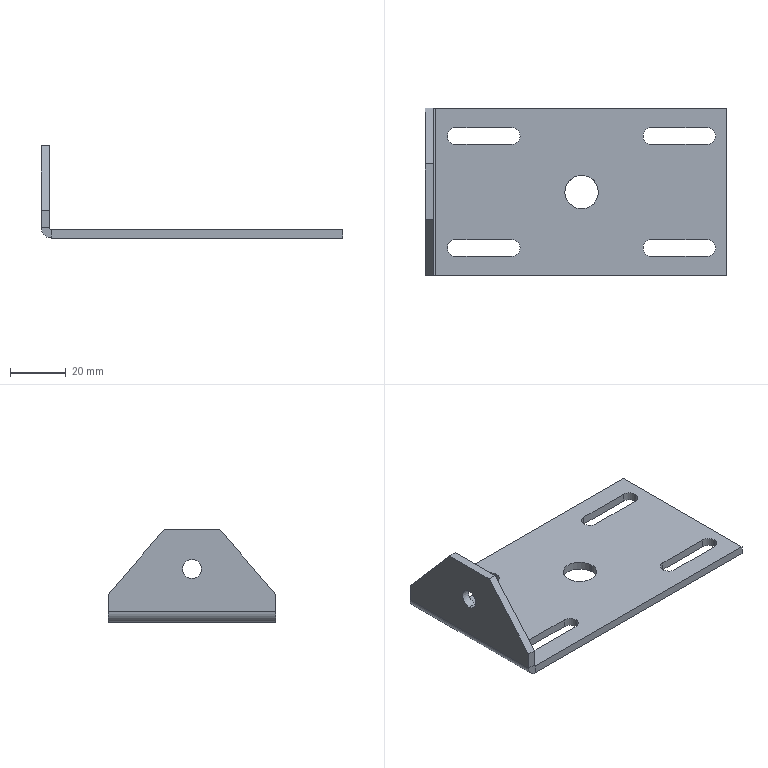Part | NX | features BREP 1 | 1 solid | 40 faces | box 108 x 60 x 33 mm | volume 21060 mm3 | plane 22 | cylinder 18 | commonest cylinder face diameters 6 x12 6.8 x2 12 x2 1.473 x1 7.473 x1
STEP:
#1=CARTESIAN_POINT('',(-48.,0.,12.6));
#2=VERTEX_POINT('',#1);
#3=CARTESIAN_POINT('',(-45.,0.,12.6));
#4=VERTEX_POINT('',#3);
#5=CARTESIAN_POINT('',(-48.,0.,12.6));
#6=DIRECTION('',(-1.,0.,0.));
#7=VECTOR('',#6,1000.);
#8=LINE('',#5,#7);
#9=EDGE_CURVE('',#2,#4,#8,.F.);
#10=ORIENTED_EDGE('',*,*,#9,.T.);
#11=CARTESIAN_POINT('',(-45.,0.,19.4));
#12=VERTEX_POINT('',#11);
#13=CARTESIAN_POINT('',(-45.,0.,16.));
#14=DIRECTION('',(1.,0.,0.));
#15=DIRECTION('',(0.,0.,-1.));
#16=AXIS2_PLACEMENT_3D('',#13,#14,#15);
#17=CIRCLE('',#16,3.4);
#18=EDGE_CURVE('',#4,#12,#17,.T.);
#19=ORIENTED_EDGE('',*,*,#18,.T.);
#20=CARTESIAN_POINT('',(-48.,0.,19.4));
#21=VERTEX_POINT('',#20);
#22=CARTESIAN_POINT('',(-48.,0.,19.4));
#23=DIRECTION('',(-1.,0.,0.));
#24=VECTOR('',#23,1000.);
#25=LINE('',#22,#24);
#26=EDGE_CURVE('',#21,#12,#25,.F.);
#27=ORIENTED_EDGE('',*,*,#26,.F.);
#28=CARTESIAN_POINT('',(-48.,0.,16.));
#29=DIRECTION('',(-1.,0.,0.));
#30=DIRECTION('',(0.,0.,1.));
#31=AXIS2_PLACEMENT_3D('',#28,#29,#30);
#32=CIRCLE('',#31,3.4);
#33=EDGE_CURVE('',#21,#2,#32,.T.);
#34=ORIENTED_EDGE('',*,*,#33,.T.);
#35=EDGE_LOOP('',(#10,#19,#27,#34));
#36=FACE_BOUND('',#35,.T.);
#37=CARTESIAN_POINT('',(-48.,0.,16.));
#38=DIRECTION('',(-1.,0.,0.));
#39=DIRECTION('',(0.,0.,1.));
#40=AXIS2_PLACEMENT_3D('',#37,#38,#39);
#41=CYLINDRICAL_SURFACE('',#40,3.4);
#42=ADVANCED_FACE('',(#36),#41,.F.);
#43=CARTESIAN_POINT('',(-17.,-17.,-3.));
#44=VERTEX_POINT('',#43);
#45=CARTESIAN_POINT('',(-17.,-17.,0.));
#46=VERTEX_POINT('',#45);
#47=CARTESIAN_POINT('',(-17.,-17.,-10.));
#48=DIRECTION('',(0.,0.,1.));
#49=VECTOR('',#48,1000.);
#50=LINE('',#47,#49);
#51=EDGE_CURVE('',#44,#46,#50,.T.);
#52=ORIENTED_EDGE('',*,*,#51,.T.);
#53=CARTESIAN_POINT('',(-37.,-17.,0.));
#54=VERTEX_POINT('',#53);
#55=CARTESIAN_POINT('',(-17.,-17.,0.));
#56=DIRECTION('',(-1.,0.,0.));
#57=VECTOR('',#56,1000.);
#58=LINE('',#55,#57);
#59=EDGE_CURVE('',#46,#54,#58,.T.);
#60=ORIENTED_EDGE('',*,*,#59,.T.);
#61=CARTESIAN_POINT('',(-37.,-17.,-3.));
#62=VERTEX_POINT('',#61);
#63=CARTESIAN_POINT('',(-37.,-17.,-10.));
#64=DIRECTION('',(0.,0.,1.));
#65=VECTOR('',#64,1000.);
#66=LINE('',#63,#65);
#67=EDGE_CURVE('',#62,#54,#66,.T.);
#68=ORIENTED_EDGE('',*,*,#67,.F.);
#69=CARTESIAN_POINT('',(0.,-17.,-3.));
#70=DIRECTION('',(-1.,0.,0.));
#71=VECTOR('',#70,1000.);
#72=LINE('',#69,#71);
#73=EDGE_CURVE('',#44,#62,#72,.T.);
#74=ORIENTED_EDGE('',*,*,#73,.F.);
#75=EDGE_LOOP('',(#52,#60,#68,#74));
#76=FACE_BOUND('',#75,.T.);
#77=CARTESIAN_POINT('',(-17.,-17.,-10.));
#78=DIRECTION('',(0.,1.,0.));
#79=DIRECTION('',(-1.,0.,0.));
#80=AXIS2_PLACEMENT_3D('',#77,#78,#79);
#81=PLANE('',#80);
#82=ADVANCED_FACE('',(#76),#81,.F.);
#83=ORIENTED_EDGE('',*,*,#67,.T.);
#84=CARTESIAN_POINT('',(-37.,-23.,0.));
#85=VERTEX_POINT('',#84);
#86=CARTESIAN_POINT('',(-37.,-20.,0.));
#87=DIRECTION('',(0.,0.,1.));
#88=DIRECTION('',(1.,0.,0.));
#89=AXIS2_PLACEMENT_3D('',#86,#87,#88);
#90=CIRCLE('',#89,3.);
#91=EDGE_CURVE('',#54,#85,#90,.T.);
#92=ORIENTED_EDGE('',*,*,#91,.T.);
#93=CARTESIAN_POINT('',(-37.,-23.,-3.));
#94=VERTEX_POINT('',#93);
#95=CARTESIAN_POINT('',(-37.,-23.,-10.));
#96=DIRECTION('',(0.,0.,1.));
#97=VECTOR('',#96,1000.);
#98=LINE('',#95,#97);
#99=EDGE_CURVE('',#94,#85,#98,.T.);
#100=ORIENTED_EDGE('',*,*,#99,.F.);
#101=CARTESIAN_POINT('',(-37.,-20.,-3.));
#102=DIRECTION('',(0.,0.,1.));
#103=DIRECTION('',(1.,0.,0.));
#104=AXIS2_PLACEMENT_3D('',#101,#102,#103);
#105=CIRCLE('',#104,3.);
#106=EDGE_CURVE('',#62,#94,#105,.T.);
#107=ORIENTED_EDGE('',*,*,#106,.F.);
#108=EDGE_LOOP('',(#83,#92,#100,#107));
#109=FACE_BOUND('',#108,.T.);
#110=CARTESIAN_POINT('',(-37.,-20.,-10.));
#111=DIRECTION('',(0.,0.,1.));
#112=DIRECTION('',(1.,0.,0.));
#113=AXIS2_PLACEMENT_3D('',#110,#111,#112);
#114=CYLINDRICAL_SURFACE('',#113,3.);
#115=ADVANCED_FACE('',(#109),#114,.F.);
#116=ORIENTED_EDGE('',*,*,#99,.T.);
#117=CARTESIAN_POINT('',(-17.,-23.,0.));
#118=VERTEX_POINT('',#117);
#119=CARTESIAN_POINT('',(-17.,-23.,0.));
#120=DIRECTION('',(1.,0.,0.));
#121=VECTOR('',#120,1000.);
#122=LINE('',#119,#121);
#123=EDGE_CURVE('',#85,#118,#122,.T.);
#124=ORIENTED_EDGE('',*,*,#123,.T.);
#125=CARTESIAN_POINT('',(-17.,-23.,-3.));
#126=VERTEX_POINT('',#125);
#127=CARTESIAN_POINT('',(-17.,-23.,-10.));
#128=DIRECTION('',(0.,0.,1.));
#129=VECTOR('',#128,1000.);
#130=LINE('',#127,#129);
#131=EDGE_CURVE('',#126,#118,#130,.T.);
#132=ORIENTED_EDGE('',*,*,#131,.F.);
#133=CARTESIAN_POINT('',(0.,-23.,-3.));
#134=DIRECTION('',(1.,0.,0.));
#135=VECTOR('',#134,1000.);
#136=LINE('',#133,#135);
#137=EDGE_CURVE('',#94,#126,#136,.T.);
#138=ORIENTED_EDGE('',*,*,#137,.F.);
#139=EDGE_LOOP('',(#116,#124,#132,#138));
#140=FACE_BOUND('',#139,.T.);
#141=CARTESIAN_POINT('',(-17.,-23.,-10.));
#142=DIRECTION('',(0.,-1.,0.));
#143=DIRECTION('',(1.,0.,0.));
#144=AXIS2_PLACEMENT_3D('',#141,#142,#143);
#145=PLANE('',#144);
#146=ADVANCED_FACE('',(#140),#145,.F.);
#147=CARTESIAN_POINT('',(-14.,-20.,-3.));
#148=VERTEX_POINT('',#147);
#149=CARTESIAN_POINT('',(-14.,-20.,0.));
#150=VERTEX_POINT('',#149);
#151=CARTESIAN_POINT('',(-14.,-20.,-10.));
#152=DIRECTION('',(0.,0.,1.));
#153=VECTOR('',#152,1000.);
#154=LINE('',#151,#153);
#155=EDGE_CURVE('',#148,#150,#154,.T.);
#156=ORIENTED_EDGE('',*,*,#155,.F.);
#157=CARTESIAN_POINT('',(-17.,-20.,-3.));
#158=DIRECTION('',(0.,0.,1.));
#159=DIRECTION('',(1.,0.,0.));
#160=AXIS2_PLACEMENT_3D('',#157,#158,#159);
#161=CIRCLE('',#160,3.);
#162=EDGE_CURVE('',#126,#148,#161,.T.);
#163=ORIENTED_EDGE('',*,*,#162,.F.);
#164=ORIENTED_EDGE('',*,*,#131,.T.);
#165=CARTESIAN_POINT('',(-17.,-20.,0.));
#166=DIRECTION('',(0.,0.,1.));
#167=DIRECTION('',(1.,0.,0.));
#168=AXIS2_PLACEMENT_3D('',#165,#166,#167);
#169=CIRCLE('',#168,3.);
#170=EDGE_CURVE('',#118,#150,#169,.T.);
#171=ORIENTED_EDGE('',*,*,#170,.T.);
#172=EDGE_LOOP('',(#156,#163,#164,#171));
#173=FACE_BOUND('',#172,.T.);
#174=CARTESIAN_POINT('',(-17.,-20.,-10.));
#175=DIRECTION('',(0.,0.,1.));
#176=DIRECTION('',(1.,0.,0.));
#177=AXIS2_PLACEMENT_3D('',#174,#175,#176);
#178=CYLINDRICAL_SURFACE('',#177,3.);
#179=ADVANCED_FACE('',(#173),#178,.F.);
#180=CARTESIAN_POINT('',(33.,-23.,-3.));
#181=VERTEX_POINT('',#180);
#182=CARTESIAN_POINT('',(33.,-23.,0.));
#183=VERTEX_POINT('',#182);
#184=CARTESIAN_POINT('',(33.,-23.,-10.));
#185=DIRECTION('',(0.,0.,1.));
#186=VECTOR('',#185,1000.);
#187=LINE('',#184,#186);
#188=EDGE_CURVE('',#181,#183,#187,.T.);
#189=ORIENTED_EDGE('',*,*,#188,.T.);
#190=CARTESIAN_POINT('',(53.,-23.,0.));
#191=VERTEX_POINT('',#190);
#192=CARTESIAN_POINT('',(33.,-23.,0.));
#193=DIRECTION('',(1.,0.,0.));
#194=VECTOR('',#193,1000.);
#195=LINE('',#192,#194);
#196=EDGE_CURVE('',#183,#191,#195,.T.);
#197=ORIENTED_EDGE('',*,*,#196,.T.);
#198=CARTESIAN_POINT('',(53.,-23.,-3.));
#199=VERTEX_POINT('',#198);
#200=CARTESIAN_POINT('',(53.,-23.,-10.));
#201=DIRECTION('',(0.,0.,1.));
#202=VECTOR('',#201,1000.);
#203=LINE('',#200,#202);
#204=EDGE_CURVE('',#199,#191,#203,.T.);
#205=ORIENTED_EDGE('',*,*,#204,.F.);
#206=CARTESIAN_POINT('',(0.,-23.,-3.));
#207=DIRECTION('',(1.,0.,0.));
#208=VECTOR('',#207,1000.);
#209=LINE('',#206,#208);
#210=EDGE_CURVE('',#181,#199,#209,.T.);
#211=ORIENTED_EDGE('',*,*,#210,.F.);
#212=EDGE_LOOP('',(#189,#197,#205,#211));
#213=FACE_BOUND('',#212,.T.);
#214=CARTESIAN_POINT('',(33.,-23.,-10.));
#215=DIRECTION('',(0.,-1.,0.));
#216=DIRECTION('',(1.,0.,0.));
#217=AXIS2_PLACEMENT_3D('',#214,#215,#216);
#218=PLANE('',#217);
#219=ADVANCED_FACE('',(#213),#218,.F.);
#220=CARTESIAN_POINT('',(56.,-20.,-3.));
#221=VERTEX_POINT('',#220);
#222=CARTESIAN_POINT('',(56.,-20.,0.));
#223=VERTEX_POINT('',#222);
#224=CARTESIAN_POINT('',(56.,-20.,-10.));
#225=DIRECTION('',(0.,0.,1.));
#226=VECTOR('',#225,1000.);
#227=LINE('',#224,#226);
#228=EDGE_CURVE('',#221,#223,#227,.T.);
#229=ORIENTED_EDGE('',*,*,#228,.F.);
#230=CARTESIAN_POINT('',(53.,-20.,-3.));
#231=DIRECTION('',(0.,0.,1.));
#232=DIRECTION('',(1.,0.,0.));
#233=AXIS2_PLACEMENT_3D('',#230,#231,#232);
#234=CIRCLE('',#233,3.);
#235=EDGE_CURVE('',#199,#221,#234,.T.);
#236=ORIENTED_EDGE('',*,*,#235,.F.);
#237=ORIENTED_EDGE('',*,*,#204,.T.);
#238=CARTESIAN_POINT('',(53.,-20.,0.));
#239=DIRECTION('',(0.,0.,1.));
#240=DIRECTION('',(1.,0.,0.));
#241=AXIS2_PLACEMENT_3D('',#238,#239,#240);
#242=CIRCLE('',#241,3.);
#243=EDGE_CURVE('',#191,#223,#242,.T.);
#244=ORIENTED_EDGE('',*,*,#243,.T.);
#245=EDGE_LOOP('',(#229,#236,#237,#244));
#246=FACE_BOUND('',#245,.T.);
#247=CARTESIAN_POINT('',(53.,-20.,-10.));
#248=DIRECTION('',(0.,0.,1.));
#249=DIRECTION('',(1.,0.,0.));
#250=AXIS2_PLACEMENT_3D('',#247,#248,#249);
#251=CYLINDRICAL_SURFACE('',#250,3.);
#252=ADVANCED_FACE('',(#246),#251,.F.);
#253=CARTESIAN_POINT('',(53.,-17.,-3.));
#254=VERTEX_POINT('',#253);
#255=CARTESIAN_POINT('',(53.,-17.,0.));
#256=VERTEX_POINT('',#255);
#257=CARTESIAN_POINT('',(53.,-17.,-10.));
#258=DIRECTION('',(0.,0.,1.));
#259=VECTOR('',#258,1000.);
#260=LINE('',#257,#259);
#261=EDGE_CURVE('',#254,#256,#260,.T.);
#262=ORIENTED_EDGE('',*,*,#261,.T.);
#263=CARTESIAN_POINT('',(33.,-17.,0.));
#264=VERTEX_POINT('',#263);
#265=CARTESIAN_POINT('',(33.,-17.,0.));
#266=DIRECTION('',(-1.,0.,0.));
#267=VECTOR('',#266,1000.);
#268=LINE('',#265,#267);
#269=EDGE_CURVE('',#256,#264,#268,.T.);
#270=ORIENTED_EDGE('',*,*,#269,.T.);
#271=CARTESIAN_POINT('',(33.,-17.,-3.));
#272=VERTEX_POINT('',#271);
#273=CARTESIAN_POINT('',(33.,-17.,-10.));
#274=DIRECTION('',(0.,0.,1.));
#275=VECTOR('',#274,1000.);
#276=LINE('',#273,#275);
#277=EDGE_CURVE('',#272,#264,#276,.T.);
#278=ORIENTED_EDGE('',*,*,#277,.F.);
#279=CARTESIAN_POINT('',(0.,-17.,-3.));
#280=DIRECTION('',(-1.,0.,0.));
#281=VECTOR('',#280,1000.);
#282=LINE('',#279,#281);
#283=EDGE_CURVE('',#254,#272,#282,.T.);
#284=ORIENTED_EDGE('',*,*,#283,.F.);
#285=EDGE_LOOP('',(#262,#270,#278,#284));
#286=FACE_BOUND('',#285,.T.);
#287=CARTESIAN_POINT('',(33.,-17.,-10.));
#288=DIRECTION('',(0.,1.,0.));
#289=DIRECTION('',(-1.,0.,0.));
#290=AXIS2_PLACEMENT_3D('',#287,#288,#289);
#291=PLANE('',#290);
#292=ADVANCED_FACE('',(#286),#291,.F.);
#293=ORIENTED_EDGE('',*,*,#277,.T.);
#294=CARTESIAN_POINT('',(33.,-20.,0.));
#295=DIRECTION('',(0.,0.,1.));
#296=DIRECTION('',(1.,0.,0.));
#297=AXIS2_PLACEMENT_3D('',#294,#295,#296);
#298=CIRCLE('',#297,3.);
#299=EDGE_CURVE('',#264,#183,#298,.T.);
#300=ORIENTED_EDGE('',*,*,#299,.T.);
#301=ORIENTED_EDGE('',*,*,#188,.F.);
#302=CARTESIAN_POINT('',(33.,-20.,-3.));
#303=DIRECTION('',(0.,0.,1.));
#304=DIRECTION('',(1.,0.,0.));
#305=AXIS2_PLACEMENT_3D('',#302,#303,#304);
#306=CIRCLE('',#305,3.);
#307=EDGE_CURVE('',#272,#181,#306,.T.);
#308=ORIENTED_EDGE('',*,*,#307,.F.);
#309=EDGE_LOOP('',(#293,#300,#301,#308));
#310=FACE_BOUND('',#309,.T.);
#311=CARTESIAN_POINT('',(33.,-20.,-10.));
#312=DIRECTION('',(0.,0.,1.));
#313=DIRECTION('',(1.,0.,0.));
#314=AXIS2_PLACEMENT_3D('',#311,#312,#313);
#315=CYLINDRICAL_SURFACE('',#314,3.);
#316=ADVANCED_FACE('',(#310),#315,.F.);
#317=CARTESIAN_POINT('',(33.,17.,-3.));
#318=VERTEX_POINT('',#317);
#319=CARTESIAN_POINT('',(33.,17.,0.));
#320=VERTEX_POINT('',#319);
#321=CARTESIAN_POINT('',(33.,17.,-10.));
#322=DIRECTION('',(0.,0.,1.));
#323=VECTOR('',#322,1000.);
#324=LINE('',#321,#323);
#325=EDGE_CURVE('',#318,#320,#324,.T.);
#326=ORIENTED_EDGE('',*,*,#325,.T.);
#327=CARTESIAN_POINT('',(53.,17.,0.));
#328=VERTEX_POINT('',#327);
#329=CARTESIAN_POINT('',(33.,17.,0.));
#330=DIRECTION('',(1.,0.,0.));
#331=VECTOR('',#330,1000.);
#332=LINE('',#329,#331);
#333=EDGE_CURVE('',#320,#328,#332,.T.);
#334=ORIENTED_EDGE('',*,*,#333,.T.);
#335=CARTESIAN_POINT('',(53.,17.,-3.));
#336=VERTEX_POINT('',#335);
#337=CARTESIAN_POINT('',(53.,17.,-10.));
#338=DIRECTION('',(0.,0.,1.));
#339=VECTOR('',#338,1000.);
#340=LINE('',#337,#339);
#341=EDGE_CURVE('',#336,#328,#340,.T.);
#342=ORIENTED_EDGE('',*,*,#341,.F.);
#343=CARTESIAN_POINT('',(0.,17.,-3.));
#344=DIRECTION('',(1.,0.,0.));
#345=VECTOR('',#344,1000.);
#346=LINE('',#343,#345);
#347=EDGE_CURVE('',#318,#336,#346,.T.);
#348=ORIENTED_EDGE('',*,*,#347,.F.);
#349=EDGE_LOOP('',(#326,#334,#342,#348));
#350=FACE_BOUND('',#349,.T.);
#351=CARTESIAN_POINT('',(33.,17.,-10.));
#352=DIRECTION('',(0.,-1.,0.));
#353=DIRECTION('',(1.,0.,0.));
#354=AXIS2_PLACEMENT_3D('',#351,#352,#353);
#355=PLANE('',#354);
#356=ADVANCED_FACE('',(#350),#355,.F.);
#357=CARTESIAN_POINT('',(56.,20.,-3.));
#358=VERTEX_POINT('',#357);
#359=CARTESIAN_POINT('',(56.,20.,0.));
#360=VERTEX_POINT('',#359);
#361=CARTESIAN_POINT('',(56.,20.,-10.));
#362=DIRECTION('',(0.,0.,1.));
#363=VECTOR('',#362,1000.);
#364=LINE('',#361,#363);
#365=EDGE_CURVE('',#358,#360,#364,.T.);
#366=ORIENTED_EDGE('',*,*,#365,.F.);
#367=CARTESIAN_POINT('',(53.,20.,-3.));
#368=DIRECTION('',(0.,0.,1.));
#369=DIRECTION('',(1.,0.,0.));
#370=AXIS2_PLACEMENT_3D('',#367,#368,#369);
#371=CIRCLE('',#370,3.);
#372=EDGE_CURVE('',#336,#358,#371,.T.);
#373=ORIENTED_EDGE('',*,*,#372,.F.);
#374=ORIENTED_EDGE('',*,*,#341,.T.);
#375=CARTESIAN_POINT('',(53.,20.,0.));
#376=DIRECTION('',(0.,0.,1.));
#377=DIRECTION('',(1.,0.,0.));
#378=AXIS2_PLACEMENT_3D('',#375,#376,#377);
#379=CIRCLE('',#378,3.);
#380=EDGE_CURVE('',#328,#360,#379,.T.);
#381=ORIENTED_EDGE('',*,*,#380,.T.);
#382=EDGE_LOOP('',(#366,#373,#374,#381));
#383=FACE_BOUND('',#382,.T.);
#384=CARTESIAN_POINT('',(53.,20.,-10.));
#385=DIRECTION('',(0.,0.,1.));
#386=DIRECTION('',(1.,0.,0.));
#387=AXIS2_PLACEMENT_3D('',#384,#385,#386);
#388=CYLINDRICAL_SURFACE('',#387,3.);
#389=ADVANCED_FACE('',(#383),#388,.F.);
#390=CARTESIAN_POINT('',(53.,23.,-3.));
#391=VERTEX_POINT('',#390);
#392=CARTESIAN_POINT('',(53.,23.,0.));
#393=VERTEX_POINT('',#392);
#394=CARTESIAN_POINT('',(53.,23.,-10.));
#395=DIRECTION('',(0.,0.,1.));
#396=VECTOR('',#395,1000.);
#397=LINE('',#394,#396);
#398=EDGE_CURVE('',#391,#393,#397,.T.);
#399=ORIENTED_EDGE('',*,*,#398,.T.);
#400=CARTESIAN_POINT('',(33.,23.,0.));
#401=VERTEX_POINT('',#400);
#402=CARTESIAN_POINT('',(33.,23.,0.));
#403=DIRECTION('',(-1.,0.,0.));
#404=VECTOR('',#403,1000.);
#405=LINE('',#402,#404);
#406=EDGE_CURVE('',#393,#401,#405,.T.);
#407=ORIENTED_EDGE('',*,*,#406,.T.);
#408=CARTESIAN_POINT('',(33.,23.,-3.));
#409=VERTEX_POINT('',#408);
#410=CARTESIAN_POINT('',(33.,23.,-10.));
#411=DIRECTION('',(0.,0.,1.));
#412=VECTOR('',#411,1000.);
#413=LINE('',#410,#412);
#414=EDGE_CURVE('',#409,#401,#413,.T.);
#415=ORIENTED_EDGE('',*,*,#414,.F.);
#416=CARTESIAN_POINT('',(0.,23.,-3.));
#417=DIRECTION('',(-1.,0.,0.));
#418=VECTOR('',#417,1000.);
#419=LINE('',#416,#418);
#420=EDGE_CURVE('',#391,#409,#419,.T.);
#421=ORIENTED_EDGE('',*,*,#420,.F.);
#422=EDGE_LOOP('',(#399,#407,#415,#421));
#423=FACE_BOUND('',#422,.T.);
#424=CARTESIAN_POINT('',(33.,23.,-10.));
#425=DIRECTION('',(0.,1.,0.));
#426=DIRECTION('',(-1.,0.,0.));
#427=AXIS2_PLACEMENT_3D('',#424,#425,#426);
#428=PLANE('',#427);
#429=ADVANCED_FACE('',(#423),#428,.F.);
#430=ORIENTED_EDGE('',*,*,#414,.T.);
#431=CARTESIAN_POINT('',(33.,20.,0.));
#432=DIRECTION('',(0.,0.,1.));
#433=DIRECTION('',(1.,0.,0.));
#434=AXIS2_PLACEMENT_3D('',#431,#432,#433);
#435=CIRCLE('',#434,3.);
#436=EDGE_CURVE('',#401,#320,#435,.T.);
#437=ORIENTED_EDGE('',*,*,#436,.T.);
#438=ORIENTED_EDGE('',*,*,#325,.F.);
#439=CARTESIAN_POINT('',(33.,20.,-3.));
#440=DIRECTION('',(0.,0.,1.));
#441=DIRECTION('',(1.,0.,0.));
#442=AXIS2_PLACEMENT_3D('',#439,#440,#441);
#443=CIRCLE('',#442,3.);
#444=EDGE_CURVE('',#409,#318,#443,.T.);
#445=ORIENTED_EDGE('',*,*,#444,.F.);
#446=EDGE_LOOP('',(#430,#437,#438,#445));
#447=FACE_BOUND('',#446,.T.);
#448=CARTESIAN_POINT('',(33.,20.,-10.));
#449=DIRECTION('',(0.,0.,1.));
#450=DIRECTION('',(1.,0.,0.));
#451=AXIS2_PLACEMENT_3D('',#448,#449,#450);
#452=CYLINDRICAL_SURFACE('',#451,3.);
#453=ADVANCED_FACE('',(#447),#452,.F.);
#454=CARTESIAN_POINT('',(-37.,17.,-3.));
#455=VERTEX_POINT('',#454);
#456=CARTESIAN_POINT('',(-37.,17.,0.));
#457=VERTEX_POINT('',#456);
#458=CARTESIAN_POINT('',(-37.,17.,-10.));
#459=DIRECTION('',(0.,0.,1.));
#460=VECTOR('',#459,1000.);
#461=LINE('',#458,#460);
#462=EDGE_CURVE('',#455,#457,#461,.T.);
#463=ORIENTED_EDGE('',*,*,#462,.T.);
#464=CARTESIAN_POINT('',(-17.,17.,0.));
#465=VERTEX_POINT('',#464);
#466=CARTESIAN_POINT('',(-37.,17.,0.));
#467=DIRECTION('',(1.,0.,0.));
#468=VECTOR('',#467,1000.);
#469=LINE('',#466,#468);
#470=EDGE_CURVE('',#457,#465,#469,.T.);
#471=ORIENTED_EDGE('',*,*,#470,.T.);
#472=CARTESIAN_POINT('',(-17.,17.,-3.));
#473=VERTEX_POINT('',#472);
#474=CARTESIAN_POINT('',(-17.,17.,-10.));
#475=DIRECTION('',(0.,0.,1.));
#476=VECTOR('',#475,1000.);
#477=LINE('',#474,#476);
#478=EDGE_CURVE('',#473,#465,#477,.T.);
#479=ORIENTED_EDGE('',*,*,#478,.F.);
#480=CARTESIAN_POINT('',(0.,17.,-3.));
#481=DIRECTION('',(1.,0.,0.));
#482=VECTOR('',#481,1000.);
#483=LINE('',#480,#482);
#484=EDGE_CURVE('',#455,#473,#483,.T.);
#485=ORIENTED_EDGE('',*,*,#484,.F.);
#486=EDGE_LOOP('',(#463,#471,#479,#485));
#487=FACE_BOUND('',#486,.T.);
#488=CARTESIAN_POINT('',(-37.,17.,-10.));
#489=DIRECTION('',(0.,-1.,0.));
#490=DIRECTION('',(0.,0.,-1.));
#491=AXIS2_PLACEMENT_3D('',#488,#489,#490);
#492=PLANE('',#491);
#493=ADVANCED_FACE('',(#487),#492,.F.);
#494=CARTESIAN_POINT('',(-14.,20.,-3.));
#495=VERTEX_POINT('',#494);
#496=CARTESIAN_POINT('',(-14.,20.,0.));
#497=VERTEX_POINT('',#496);
#498=CARTESIAN_POINT('',(-14.,20.,-10.));
#499=DIRECTION('',(0.,0.,1.));
#500=VECTOR('',#499,1000.);
#501=LINE('',#498,#500);
#502=EDGE_CURVE('',#495,#497,#501,.T.);
#503=ORIENTED_EDGE('',*,*,#502,.F.);
#504=CARTESIAN_POINT('',(-17.,20.,-3.));
#505=DIRECTION('',(0.,0.,1.));
#506=DIRECTION('',(1.,0.,0.));
#507=AXIS2_PLACEMENT_3D('',#504,#505,#506);
#508=CIRCLE('',#507,3.);
#509=EDGE_CURVE('',#473,#495,#508,.T.);
#510=ORIENTED_EDGE('',*,*,#509,.F.);
#511=ORIENTED_EDGE('',*,*,#478,.T.);
#512=CARTESIAN_POINT('',(-17.,20.,0.));
#513=DIRECTION('',(0.,0.,1.));
#514=DIRECTION('',(1.,0.,0.));
#515=AXIS2_PLACEMENT_3D('',#512,#513,#514);
#516=CIRCLE('',#515,3.);
#517=EDGE_CURVE('',#465,#497,#516,.T.);
#518=ORIENTED_EDGE('',*,*,#517,.T.);
#519=EDGE_LOOP('',(#503,#510,#511,#518));
#520=FACE_BOUND('',#519,.T.);
#521=CARTESIAN_POINT('',(-17.,20.,-10.));
#522=DIRECTION('',(0.,0.,1.));
#523=DIRECTION('',(1.,0.,0.));
#524=AXIS2_PLACEMENT_3D('',#521,#522,#523);
#525=CYLINDRICAL_SURFACE('',#524,3.);
#526=ADVANCED_FACE('',(#520),#525,.F.);
#527=CARTESIAN_POINT('',(-17.,23.,-3.));
#528=VERTEX_POINT('',#527);
#529=CARTESIAN_POINT('',(-17.,23.,0.));
#530=VERTEX_POINT('',#529);
#531=CARTESIAN_POINT('',(-17.,23.,-10.));
#532=DIRECTION('',(0.,0.,1.));
#533=VECTOR('',#532,1000.);
#534=LINE('',#531,#533);
#535=EDGE_CURVE('',#528,#530,#534,.T.);
#536=ORIENTED_EDGE('',*,*,#535,.T.);
#537=CARTESIAN_POINT('',(-37.,23.,0.));
#538=VERTEX_POINT('',#537);
#539=CARTESIAN_POINT('',(-37.,23.,0.));
#540=DIRECTION('',(-1.,0.,0.));
#541=VECTOR('',#540,1000.);
#542=LINE('',#539,#541);
#543=EDGE_CURVE('',#530,#538,#542,.T.);
#544=ORIENTED_EDGE('',*,*,#543,.T.);
#545=CARTESIAN_POINT('',(-37.,23.,-3.));
#546=VERTEX_POINT('',#545);
#547=CARTESIAN_POINT('',(-37.,23.,-10.));
#548=DIRECTION('',(0.,0.,1.));
#549=VECTOR('',#548,1000.);
#550=LINE('',#547,#549);
#551=EDGE_CURVE('',#546,#538,#550,.T.);
#552=ORIENTED_EDGE('',*,*,#551,.F.);
#553=CARTESIAN_POINT('',(0.,23.,-3.));
#554=DIRECTION('',(-1.,0.,0.));
#555=VECTOR('',#554,1000.);
#556=LINE('',#553,#555);
#557=EDGE_CURVE('',#528,#546,#556,.T.);
#558=ORIENTED_EDGE('',*,*,#557,.F.);
#559=EDGE_LOOP('',(#536,#544,#552,#558));
#560=FACE_BOUND('',#559,.T.);
#561=CARTESIAN_POINT('',(-37.,23.,-10.));
#562=DIRECTION('',(0.,1.,0.));
#563=DIRECTION('',(0.,0.,1.));
#564=AXIS2_PLACEMENT_3D('',#561,#562,#563);
#565=PLANE('',#564);
#566=ADVANCED_FACE('',(#560),#565,.F.);
#567=ORIENTED_EDGE('',*,*,#551,.T.);
#568=CARTESIAN_POINT('',(-37.,20.,0.));
#569=DIRECTION('',(0.,0.,1.));
#570=DIRECTION('',(1.,0.,0.));
#571=AXIS2_PLACEMENT_3D('',#568,#569,#570);
#572=CIRCLE('',#571,3.);
#573=EDGE_CURVE('',#538,#457,#572,.T.);
#574=ORIENTED_EDGE('',*,*,#573,.T.);
#575=ORIENTED_EDGE('',*,*,#462,.F.);
#576=CARTESIAN_POINT('',(-37.,20.,-3.));
#577=DIRECTION('',(0.,0.,1.));
#578=DIRECTION('',(1.,0.,0.));
#579=AXIS2_PLACEMENT_3D('',#576,#577,#578);
#580=CIRCLE('',#579,3.);
#581=EDGE_CURVE('',#546,#455,#580,.T.);
#582=ORIENTED_EDGE('',*,*,#581,.F.);
#583=EDGE_LOOP('',(#567,#574,#575,#582));
#584=FACE_BOUND('',#583,.T.);
#585=CARTESIAN_POINT('',(-37.,20.,-10.));
#586=DIRECTION('',(0.,0.,1.));
#587=DIRECTION('',(1.,0.,0.));
#588=AXIS2_PLACEMENT_3D('',#585,#586,#587);
#589=CYLINDRICAL_SURFACE('',#588,3.);
#590=ADVANCED_FACE('',(#584),#589,.F.);
#591=CARTESIAN_POINT('',(-45.,10.,30.));
#592=VERTEX_POINT('',#591);
#593=CARTESIAN_POINT('',(-45.,30.,7.));
#594=VERTEX_POINT('',#593);
#595=CARTESIAN_POINT('',(-45.,20.549,17.869));
#596=DIRECTION('',(0.,0.6562,-0.7546));
#597=VECTOR('',#596,1000.);
#598=LINE('',#595,#597);
#599=EDGE_CURVE('',#592,#594,#598,.T.);
#600=ORIENTED_EDGE('',*,*,#599,.T.);
#601=CARTESIAN_POINT('',(-48.,30.,7.));
#602=VERTEX_POINT('',#601);
#603=CARTESIAN_POINT('',(-45.,30.,7.));
#604=DIRECTION('',(-1.,0.,0.));
#605=VECTOR('',#604,1000.);
#606=LINE('',#603,#605);
#607=EDGE_CURVE('',#594,#602,#606,.T.);
#608=ORIENTED_EDGE('',*,*,#607,.T.);
#609=CARTESIAN_POINT('',(-48.,10.,30.));
#610=VERTEX_POINT('',#609);
#611=CARTESIAN_POINT('',(-48.,20.549,17.869));
#612=DIRECTION('',(0.,0.6562,-0.7546));
#613=VECTOR('',#612,1000.);
#614=LINE('',#611,#613);
#615=EDGE_CURVE('',#610,#602,#614,.T.);
#616=ORIENTED_EDGE('',*,*,#615,.F.);
#617=CARTESIAN_POINT('',(-45.,10.,30.));
#618=DIRECTION('',(-1.,0.,0.));
#619=VECTOR('',#618,1000.);
#620=LINE('',#617,#619);
#621=EDGE_CURVE('',#592,#610,#620,.T.);
#622=ORIENTED_EDGE('',*,*,#621,.F.);
#623=EDGE_LOOP('',(#600,#608,#616,#622));
#624=FACE_BOUND('',#623,.T.);
#625=CARTESIAN_POINT('',(-45.,20.549,17.869));
#626=DIRECTION('',(0.,-0.7546,-0.6562));
#627=DIRECTION('',(0.,0.6562,-0.7546));
#628=AXIS2_PLACEMENT_3D('',#625,#626,#627);
#629=PLANE('',#628);
#630=ADVANCED_FACE('',(#624),#629,.F.);
#631=CARTESIAN_POINT('',(-45.,-30.,7.));
#632=VERTEX_POINT('',#631);
#633=CARTESIAN_POINT('',(-45.,-10.,30.));
#634=VERTEX_POINT('',#633);
#635=CARTESIAN_POINT('',(-45.,-20.549,17.869));
#636=DIRECTION('',(0.,0.6562,0.7546));
#637=VECTOR('',#636,1000.);
#638=LINE('',#635,#637);
#639=EDGE_CURVE('',#632,#634,#638,.T.);
#640=ORIENTED_EDGE('',*,*,#639,.T.);
#641=CARTESIAN_POINT('',(-48.,-10.,30.));
#642=VERTEX_POINT('',#641);
#643=CARTESIAN_POINT('',(-45.,-10.,30.));
#644=DIRECTION('',(-1.,0.,0.));
#645=VECTOR('',#644,1000.);
#646=LINE('',#643,#645);
#647=EDGE_CURVE('',#634,#642,#646,.T.);
#648=ORIENTED_EDGE('',*,*,#647,.T.);
#649=CARTESIAN_POINT('',(-48.,-30.,7.));
#650=VERTEX_POINT('',#649);
#651=CARTESIAN_POINT('',(-48.,-20.549,17.869));
#652=DIRECTION('',(0.,0.6562,0.7546));
#653=VECTOR('',#652,1000.);
#654=LINE('',#651,#653);
#655=EDGE_CURVE('',#650,#642,#654,.T.);
#656=ORIENTED_EDGE('',*,*,#655,.F.);
#657=CARTESIAN_POINT('',(-45.,-30.,7.));
#658=DIRECTION('',(-1.,0.,0.));
#659=VECTOR('',#658,1000.);
#660=LINE('',#657,#659);
#661=EDGE_CURVE('',#632,#650,#660,.T.);
#662=ORIENTED_EDGE('',*,*,#661,.F.);
#663=EDGE_LOOP('',(#640,#648,#656,#662));
#664=FACE_BOUND('',#663,.T.);
#665=CARTESIAN_POINT('',(-45.,-20.549,17.869));
#666=DIRECTION('',(0.,0.7546,-0.6562));
#667=DIRECTION('',(0.,0.6562,0.7546));
#668=AXIS2_PLACEMENT_3D('',#665,#666,#667);
#669=PLANE('',#668);
#670=ADVANCED_FACE('',(#664),#669,.F.);
#671=CARTESIAN_POINT('',(2.,0.,0.));
#672=VERTEX_POINT('',#671);
#673=CARTESIAN_POINT('',(2.,0.,-3.));
#674=VERTEX_POINT('',#673);
#675=CARTESIAN_POINT('',(2.,0.,-10.));
#676=DIRECTION('',(0.,0.,1.));
#677=VECTOR('',#676,1000.);
#678=LINE('',#675,#677);
#679=EDGE_CURVE('',#672,#674,#678,.F.);
#680=ORIENTED_EDGE('',*,*,#679,.T.);
#681=CARTESIAN_POINT('',(14.,0.,-3.));
#682=VERTEX_POINT('',#681);
#683=CARTESIAN_POINT('',(8.,0.,-3.));
#684=DIRECTION('',(0.,0.,1.));
#685=DIRECTION('',(1.,0.,0.));
#686=AXIS2_PLACEMENT_3D('',#683,#684,#685);
#687=CIRCLE('',#686,6.);
#688=EDGE_CURVE('',#682,#674,#687,.T.);
#689=ORIENTED_EDGE('',*,*,#688,.F.);
#690=CARTESIAN_POINT('',(14.,0.,0.));
#691=VERTEX_POINT('',#690);
#692=CARTESIAN_POINT('',(14.,0.,-10.));
#693=DIRECTION('',(0.,0.,1.));
#694=VECTOR('',#693,1000.);
#695=LINE('',#692,#694);
#696=EDGE_CURVE('',#691,#682,#695,.F.);
#697=ORIENTED_EDGE('',*,*,#696,.F.);
#698=CARTESIAN_POINT('',(8.,0.,0.));
#699=DIRECTION('',(0.,0.,1.));
#700=DIRECTION('',(1.,0.,0.));
#701=AXIS2_PLACEMENT_3D('',#698,#699,#700);
#702=CIRCLE('',#701,6.);
#703=EDGE_CURVE('',#691,#672,#702,.T.);
#704=ORIENTED_EDGE('',*,*,#703,.T.);
#705=EDGE_LOOP('',(#680,#689,#697,#704));
#706=FACE_BOUND('',#705,.T.);
#707=CARTESIAN_POINT('',(8.,0.,-10.));
#708=DIRECTION('',(0.,0.,1.));
#709=DIRECTION('',(1.,0.,0.));
#710=AXIS2_PLACEMENT_3D('',#707,#708,#709);
#711=CYLINDRICAL_SURFACE('',#710,6.);
#712=ADVANCED_FACE('',(#706),#711,.F.);
#713=CARTESIAN_POINT('',(-44.263,-30.,0.));
#714=VERTEX_POINT('',#713);
#715=CARTESIAN_POINT('',(-44.263,30.,0.));
#716=VERTEX_POINT('',#715);
#717=CARTESIAN_POINT('',(-44.263,-30.,0.));
#718=DIRECTION('',(0.,1.,0.));
#719=VECTOR('',#718,1000.);
#720=LINE('',#717,#719);
#721=EDGE_CURVE('',#714,#716,#720,.T.);
#722=ORIENTED_EDGE('',*,*,#721,.T.);
#723=CARTESIAN_POINT('',(-45.,30.,0.7366));
#724=VERTEX_POINT('',#723);
#725=CARTESIAN_POINT('',(-44.263,30.,0.7366));
#726=DIRECTION('',(0.,1.,0.));
#727=DIRECTION('',(0.,0.,-1.));
#728=AXIS2_PLACEMENT_3D('',#725,#726,#727);
#729=CIRCLE('',#728,0.7366);
#730=EDGE_CURVE('',#716,#724,#729,.T.);
#731=ORIENTED_EDGE('',*,*,#730,.T.);
#732=CARTESIAN_POINT('',(-45.,-30.,0.7366));
#733=VERTEX_POINT('',#732);
#734=CARTESIAN_POINT('',(-45.,30.,0.7366));
#735=DIRECTION('',(0.,-1.,0.));
#736=VECTOR('',#735,1000.);
#737=LINE('',#734,#736);
#738=EDGE_CURVE('',#724,#733,#737,.T.);
#739=ORIENTED_EDGE('',*,*,#738,.T.);
#740=CARTESIAN_POINT('',(-44.263,-30.,0.7366));
#741=DIRECTION('',(0.,-1.,0.));
#742=DIRECTION('',(0.,0.,-1.));
#743=AXIS2_PLACEMENT_3D('',#740,#741,#742);
#744=CIRCLE('',#743,0.7366);
#745=EDGE_CURVE('',#733,#714,#744,.T.);
#746=ORIENTED_EDGE('',*,*,#745,.T.);
#747=EDGE_LOOP('',(#722,#731,#739,#746));
#748=FACE_BOUND('',#747,.T.);
#749=CARTESIAN_POINT('',(-44.263,-30.,0.7366));
#750=DIRECTION('',(0.,-1.,0.));
#751=DIRECTION('',(-1.,0.,0.));
#752=AXIS2_PLACEMENT_3D('',#749,#750,#751);
#753=CYLINDRICAL_SURFACE('',#752,0.7366);
#754=ADVANCED_FACE('',(#748),#753,.F.);
#755=CARTESIAN_POINT('',(-44.263,-30.,-3.));
#756=VERTEX_POINT('',#755);
#757=CARTESIAN_POINT('',(-44.263,30.,-3.));
#758=VERTEX_POINT('',#757);
#759=CARTESIAN_POINT('',(-44.263,-30.,-3.));
#760=DIRECTION('',(0.,1.,0.));
#761=VECTOR('',#760,1000.);
#762=LINE('',#759,#761);
#763=EDGE_CURVE('',#756,#758,#762,.T.);
#764=ORIENTED_EDGE('',*,*,#763,.F.);
#765=CARTESIAN_POINT('',(-48.,-30.,0.7366));
#766=VERTEX_POINT('',#765);
#767=CARTESIAN_POINT('',(-44.263,-30.,0.7366));
#768=DIRECTION('',(0.,-1.,0.));
#769=DIRECTION('',(0.,0.,-1.));
#770=AXIS2_PLACEMENT_3D('',#767,#768,#769);
#771=CIRCLE('',#770,3.737);
#772=EDGE_CURVE('',#766,#756,#771,.T.);
#773=ORIENTED_EDGE('',*,*,#772,.F.);
#774=CARTESIAN_POINT('',(-48.,30.,0.7366));
#775=VERTEX_POINT('',#774);
#776=CARTESIAN_POINT('',(-48.,0.,0.7366));
#777=DIRECTION('',(0.,1.,0.));
#778=VECTOR('',#777,1000.);
#779=LINE('',#776,#778);
#780=EDGE_CURVE('',#766,#775,#779,.T.);
#781=ORIENTED_EDGE('',*,*,#780,.T.);
#782=CARTESIAN_POINT('',(-44.263,30.,0.7366));
#783=DIRECTION('',(0.,1.,0.));
#784=DIRECTION('',(0.,0.,-1.));
#785=AXIS2_PLACEMENT_3D('',#782,#783,#784);
#786=CIRCLE('',#785,3.737);
#787=EDGE_CURVE('',#758,#775,#786,.T.);
#788=ORIENTED_EDGE('',*,*,#787,.F.);
#789=EDGE_LOOP('',(#764,#773,#781,#788));
#790=FACE_BOUND('',#789,.T.);
#791=CARTESIAN_POINT('',(-44.263,-30.,0.7366));
#792=DIRECTION('',(0.,-1.,0.));
#793=DIRECTION('',(-1.,0.,0.));
#794=AXIS2_PLACEMENT_3D('',#791,#792,#793);
#795=CYLINDRICAL_SURFACE('',#794,3.737);
#796=ADVANCED_FACE('',(#790),#795,.T.);
#797=ORIENTED_EDGE('',*,*,#745,.F.);
#798=CARTESIAN_POINT('',(-45.,-30.,0.7366));
#799=DIRECTION('',(-1.,0.,0.));
#800=VECTOR('',#799,1000.);
#801=LINE('',#798,#800);
#802=EDGE_CURVE('',#733,#766,#801,.T.);
#803=ORIENTED_EDGE('',*,*,#802,.T.);
#804=ORIENTED_EDGE('',*,*,#772,.T.);
#805=CARTESIAN_POINT('',(-44.263,-30.,0.));
#806=DIRECTION('',(0.,0.,-1.));
#807=VECTOR('',#806,1000.);
#808=LINE('',#805,#807);
#809=EDGE_CURVE('',#714,#756,#808,.T.);
#810=ORIENTED_EDGE('',*,*,#809,.F.);
#811=EDGE_LOOP('',(#797,#803,#804,#810));
#812=FACE_BOUND('',#811,.T.);
#813=CARTESIAN_POINT('',(-44.263,-30.,0.7366));
#814=DIRECTION('',(0.,1.,0.));
#815=DIRECTION('',(0.,0.,1.));
#816=AXIS2_PLACEMENT_3D('',#813,#814,#815);
#817=PLANE('',#816);
#818=ADVANCED_FACE('',(#812),#817,.F.);
#819=CARTESIAN_POINT('',(-45.,30.,0.7366));
#820=DIRECTION('',(-1.,0.,0.));
#821=VECTOR('',#820,1000.);
#822=LINE('',#819,#821);
#823=EDGE_CURVE('',#724,#775,#822,.T.);
#824=ORIENTED_EDGE('',*,*,#823,.F.);
#825=ORIENTED_EDGE('',*,*,#730,.F.);
#826=CARTESIAN_POINT('',(-44.263,30.,0.));
#827=DIRECTION('',(0.,0.,-1.));
#828=VECTOR('',#827,1000.);
#829=LINE('',#826,#828);
#830=EDGE_CURVE('',#716,#758,#829,.T.);
#831=ORIENTED_EDGE('',*,*,#830,.T.);
#832=ORIENTED_EDGE('',*,*,#787,.T.);
#833=EDGE_LOOP('',(#824,#825,#831,#832));
#834=FACE_BOUND('',#833,.T.);
#835=CARTESIAN_POINT('',(-44.263,30.,0.7366));
#836=DIRECTION('',(0.,1.,0.));
#837=DIRECTION('',(0.,0.,1.));
#838=AXIS2_PLACEMENT_3D('',#835,#836,#837);
#839=PLANE('',#838);
#840=ADVANCED_FACE('',(#834),#839,.T.);
#841=CARTESIAN_POINT('',(60.,-30.,0.));
#842=VERTEX_POINT('',#841);
#843=CARTESIAN_POINT('',(60.,30.,0.));
#844=VERTEX_POINT('',#843);
#845=CARTESIAN_POINT('',(60.,30.,0.));
#846=DIRECTION('',(0.,1.,0.));
#847=VECTOR('',#846,1000.);
#848=LINE('',#845,#847);
#849=EDGE_CURVE('',#842,#844,#848,.T.);
#850=ORIENTED_EDGE('',*,*,#849,.F.);
#851=CARTESIAN_POINT('',(60.,-30.,-3.));
#852=VERTEX_POINT('',#851);
#853=CARTESIAN_POINT('',(60.,-30.,-3.));
#854=DIRECTION('',(0.,0.,1.));
#855=VECTOR('',#854,1000.);
#856=LINE('',#853,#855);
#857=EDGE_CURVE('',#852,#842,#856,.T.);
#858=ORIENTED_EDGE('',*,*,#857,.F.);
#859=CARTESIAN_POINT('',(60.,30.,-3.));
#860=VERTEX_POINT('',#859);
#861=CARTESIAN_POINT('',(60.,30.,-3.));
#862=DIRECTION('',(0.,1.,0.));
#863=VECTOR('',#862,1000.);
#864=LINE('',#861,#863);
#865=EDGE_CURVE('',#852,#860,#864,.T.);
#866=ORIENTED_EDGE('',*,*,#865,.T.);
#867=CARTESIAN_POINT('',(60.,30.,-3.));
#868=DIRECTION('',(0.,0.,1.));
#869=VECTOR('',#868,1000.);
#870=LINE('',#867,#869);
#871=EDGE_CURVE('',#860,#844,#870,.T.);
#872=ORIENTED_EDGE('',*,*,#871,.T.);
#873=EDGE_LOOP('',(#850,#858,#866,#872));
#874=FACE_BOUND('',#873,.T.);
#875=CARTESIAN_POINT('',(60.,30.,-3.));
#876=DIRECTION('',(1.,0.,0.));
#877=DIRECTION('',(0.,1.,0.));
#878=AXIS2_PLACEMENT_3D('',#875,#876,#877);
#879=PLANE('',#878);
#880=ADVANCED_FACE('',(#874),#879,.T.);
#881=ORIENTED_EDGE('',*,*,#830,.F.);
#882=CARTESIAN_POINT('',(-45.,30.,0.));
#883=DIRECTION('',(-1.,0.,0.));
#884=VECTOR('',#883,1000.);
#885=LINE('',#882,#884);
#886=EDGE_CURVE('',#844,#716,#885,.T.);
#887=ORIENTED_EDGE('',*,*,#886,.F.);
#888=ORIENTED_EDGE('',*,*,#871,.F.);
#889=CARTESIAN_POINT('',(-45.,30.,-3.));
#890=DIRECTION('',(-1.,0.,0.));
#891=VECTOR('',#890,1000.);
#892=LINE('',#889,#891);
#893=EDGE_CURVE('',#860,#758,#892,.T.);
#894=ORIENTED_EDGE('',*,*,#893,.T.);
#895=EDGE_LOOP('',(#881,#887,#888,#894));
#896=FACE_BOUND('',#895,.T.);
#897=CARTESIAN_POINT('',(-45.,30.,-3.));
#898=DIRECTION('',(0.,1.,0.));
#899=DIRECTION('',(0.,0.,1.));
#900=AXIS2_PLACEMENT_3D('',#897,#898,#899);
#901=PLANE('',#900);
#902=ADVANCED_FACE('',(#896),#901,.T.);
#903=ORIENTED_EDGE('',*,*,#886,.T.);
#904=ORIENTED_EDGE('',*,*,#721,.F.);
#905=CARTESIAN_POINT('',(-45.,-30.,0.));
#906=DIRECTION('',(1.,0.,0.));
#907=VECTOR('',#906,1000.);
#908=LINE('',#905,#907);
#909=EDGE_CURVE('',#714,#842,#908,.T.);
#910=ORIENTED_EDGE('',*,*,#909,.T.);
#911=ORIENTED_EDGE('',*,*,#849,.T.);
#912=EDGE_LOOP('',(#903,#904,#910,#911));
#913=FACE_BOUND('',#912,.T.);
#914=ORIENTED_EDGE('',*,*,#703,.F.);
#915=CARTESIAN_POINT('',(8.,0.,0.));
#916=DIRECTION('',(0.,0.,1.));
#917=DIRECTION('',(1.,0.,0.));
#918=AXIS2_PLACEMENT_3D('',#915,#916,#917);
#919=CIRCLE('',#918,6.);
#920=EDGE_CURVE('',#672,#691,#919,.T.);
#921=ORIENTED_EDGE('',*,*,#920,.F.);
#922=EDGE_LOOP('',(#914,#921));
#923=FACE_BOUND('',#922,.T.);
#924=ORIENTED_EDGE('',*,*,#573,.F.);
#925=ORIENTED_EDGE('',*,*,#543,.F.);
#926=CARTESIAN_POINT('',(-17.,20.,0.));
#927=DIRECTION('',(0.,0.,1.));
#928=DIRECTION('',(1.,0.,0.));
#929=AXIS2_PLACEMENT_3D('',#926,#927,#928);
#930=CIRCLE('',#929,3.);
#931=EDGE_CURVE('',#497,#530,#930,.T.);
#932=ORIENTED_EDGE('',*,*,#931,.F.);
#933=ORIENTED_EDGE('',*,*,#517,.F.);
#934=ORIENTED_EDGE('',*,*,#470,.F.);
#935=EDGE_LOOP('',(#924,#925,#932,#933,#934));
#936=FACE_BOUND('',#935,.T.);
#937=ORIENTED_EDGE('',*,*,#436,.F.);
#938=ORIENTED_EDGE('',*,*,#406,.F.);
#939=CARTESIAN_POINT('',(53.,20.,0.));
#940=DIRECTION('',(0.,0.,1.));
#941=DIRECTION('',(1.,0.,0.));
#942=AXIS2_PLACEMENT_3D('',#939,#940,#941);
#943=CIRCLE('',#942,3.);
#944=EDGE_CURVE('',#360,#393,#943,.T.);
#945=ORIENTED_EDGE('',*,*,#944,.F.);
#946=ORIENTED_EDGE('',*,*,#380,.F.);
#947=ORIENTED_EDGE('',*,*,#333,.F.);
#948=EDGE_LOOP('',(#937,#938,#945,#946,#947));
#949=FACE_BOUND('',#948,.T.);
#950=ORIENTED_EDGE('',*,*,#299,.F.);
#951=ORIENTED_EDGE('',*,*,#269,.F.);
#952=CARTESIAN_POINT('',(53.,-20.,0.));
#953=DIRECTION('',(0.,0.,1.));
#954=DIRECTION('',(1.,0.,0.));
#955=AXIS2_PLACEMENT_3D('',#952,#953,#954);
#956=CIRCLE('',#955,3.);
#957=EDGE_CURVE('',#223,#256,#956,.T.);
#958=ORIENTED_EDGE('',*,*,#957,.F.);
#959=ORIENTED_EDGE('',*,*,#243,.F.);
#960=ORIENTED_EDGE('',*,*,#196,.F.);
#961=EDGE_LOOP('',(#950,#951,#958,#959,#960));
#962=FACE_BOUND('',#961,.T.);
#963=ORIENTED_EDGE('',*,*,#170,.F.);
#964=ORIENTED_EDGE('',*,*,#123,.F.);
#965=ORIENTED_EDGE('',*,*,#91,.F.);
#966=ORIENTED_EDGE('',*,*,#59,.F.);
#967=CARTESIAN_POINT('',(-17.,-20.,0.));
#968=DIRECTION('',(0.,0.,1.));
#969=DIRECTION('',(1.,0.,0.));
#970=AXIS2_PLACEMENT_3D('',#967,#968,#969);
#971=CIRCLE('',#970,3.);
#972=EDGE_CURVE('',#150,#46,#971,.T.);
#973=ORIENTED_EDGE('',*,*,#972,.F.);
#974=EDGE_LOOP('',(#963,#964,#965,#966,#973));
#975=FACE_BOUND('',#974,.T.);
#976=CARTESIAN_POINT('',(0.,0.,0.));
#977=DIRECTION('',(0.,0.,1.));
#978=DIRECTION('',(1.,0.,0.));
#979=AXIS2_PLACEMENT_3D('',#976,#977,#978);
#980=PLANE('',#979);
#981=ADVANCED_FACE('',(#913,#923,#936,#949,#962,#975),#980,.T.);
#982=ORIENTED_EDGE('',*,*,#763,.T.);
#983=ORIENTED_EDGE('',*,*,#893,.F.);
#984=ORIENTED_EDGE('',*,*,#865,.F.);
#985=CARTESIAN_POINT('',(-45.,-30.,-3.));
#986=DIRECTION('',(1.,0.,0.));
#987=VECTOR('',#986,1000.);
#988=LINE('',#985,#987);
#989=EDGE_CURVE('',#756,#852,#988,.T.);
#990=ORIENTED_EDGE('',*,*,#989,.F.);
#991=EDGE_LOOP('',(#982,#983,#984,#990));
#992=FACE_BOUND('',#991,.T.);
#993=ORIENTED_EDGE('',*,*,#688,.T.);
#994=CARTESIAN_POINT('',(8.,0.,-3.));
#995=DIRECTION('',(0.,0.,1.));
#996=DIRECTION('',(1.,0.,0.));
#997=AXIS2_PLACEMENT_3D('',#994,#995,#996);
#998=CIRCLE('',#997,6.);
#999=EDGE_CURVE('',#674,#682,#998,.T.);
#1000=ORIENTED_EDGE('',*,*,#999,.T.);
#1001=EDGE_LOOP('',(#993,#1000));
#1002=FACE_BOUND('',#1001,.T.);
#1003=ORIENTED_EDGE('',*,*,#557,.T.);
#1004=ORIENTED_EDGE('',*,*,#581,.T.);
#1005=ORIENTED_EDGE('',*,*,#484,.T.);
#1006=ORIENTED_EDGE('',*,*,#509,.T.);
#1007=CARTESIAN_POINT('',(-17.,20.,-3.));
#1008=DIRECTION('',(0.,0.,1.));
#1009=DIRECTION('',(1.,0.,0.));
#1010=AXIS2_PLACEMENT_3D('',#1007,#1008,#1009);
#1011=CIRCLE('',#1010,3.);
#1012=EDGE_CURVE('',#495,#528,#1011,.T.);
#1013=ORIENTED_EDGE('',*,*,#1012,.T.);
#1014=EDGE_LOOP('',(#1003,#1004,#1005,#1006,#1013));
#1015=FACE_BOUND('',#1014,.T.);
#1016=ORIENTED_EDGE('',*,*,#420,.T.);
#1017=ORIENTED_EDGE('',*,*,#444,.T.);
#1018=ORIENTED_EDGE('',*,*,#347,.T.);
#1019=ORIENTED_EDGE('',*,*,#372,.T.);
#1020=CARTESIAN_POINT('',(53.,20.,-3.));
#1021=DIRECTION('',(0.,0.,1.));
#1022=DIRECTION('',(1.,0.,0.));
#1023=AXIS2_PLACEMENT_3D('',#1020,#1021,#1022);
#1024=CIRCLE('',#1023,3.);
#1025=EDGE_CURVE('',#358,#391,#1024,.T.);
#1026=ORIENTED_EDGE('',*,*,#1025,.T.);
#1027=EDGE_LOOP('',(#1016,#1017,#1018,#1019,#1026));
#1028=FACE_BOUND('',#1027,.T.);
#1029=ORIENTED_EDGE('',*,*,#283,.T.);
#1030=ORIENTED_EDGE('',*,*,#307,.T.);
#1031=ORIENTED_EDGE('',*,*,#210,.T.);
#1032=ORIENTED_EDGE('',*,*,#235,.T.);
#1033=CARTESIAN_POINT('',(53.,-20.,-3.));
#1034=DIRECTION('',(0.,0.,1.));
#1035=DIRECTION('',(1.,0.,0.));
#1036=AXIS2_PLACEMENT_3D('',#1033,#1034,#1035);
#1037=CIRCLE('',#1036,3.);
#1038=EDGE_CURVE('',#221,#254,#1037,.T.);
#1039=ORIENTED_EDGE('',*,*,#1038,.T.);
#1040=EDGE_LOOP('',(#1029,#1030,#1031,#1032,#1039));
#1041=FACE_BOUND('',#1040,.T.);
#1042=ORIENTED_EDGE('',*,*,#137,.T.);
#1043=ORIENTED_EDGE('',*,*,#162,.T.);
#1044=CARTESIAN_POINT('',(-17.,-20.,-3.));
#1045=DIRECTION('',(0.,0.,1.));
#1046=DIRECTION('',(1.,0.,0.));
#1047=AXIS2_PLACEMENT_3D('',#1044,#1045,#1046);
#1048=CIRCLE('',#1047,3.);
#1049=EDGE_CURVE('',#148,#44,#1048,.T.);
#1050=ORIENTED_EDGE('',*,*,#1049,.T.);
#1051=ORIENTED_EDGE('',*,*,#73,.T.);
#1052=ORIENTED_EDGE('',*,*,#106,.T.);
#1053=EDGE_LOOP('',(#1042,#1043,#1050,#1051,#1052));
#1054=FACE_BOUND('',#1053,.T.);
#1055=CARTESIAN_POINT('',(0.,0.,-3.));
#1056=DIRECTION('',(0.,0.,1.));
#1057=DIRECTION('',(1.,0.,0.));
#1058=AXIS2_PLACEMENT_3D('',#1055,#1056,#1057);
#1059=PLANE('',#1058);
#1060=ADVANCED_FACE('',(#992,#1002,#1015,#1028,#1041,#1054),#1059,.F.);
#1061=ORIENTED_EDGE('',*,*,#909,.F.);
#1062=ORIENTED_EDGE('',*,*,#809,.T.);
#1063=ORIENTED_EDGE('',*,*,#989,.T.);
#1064=ORIENTED_EDGE('',*,*,#857,.T.);
#1065=EDGE_LOOP('',(#1061,#1062,#1063,#1064));
#1066=FACE_BOUND('',#1065,.T.);
#1067=CARTESIAN_POINT('',(-45.,-30.,-3.));
#1068=DIRECTION('',(0.,-1.,0.));
#1069=DIRECTION('',(0.,0.,-1.));
#1070=AXIS2_PLACEMENT_3D('',#1067,#1068,#1069);
#1071=PLANE('',#1070);
#1072=ADVANCED_FACE('',(#1066),#1071,.T.);
#1073=ORIENTED_EDGE('',*,*,#661,.T.);
#1074=CARTESIAN_POINT('',(-48.,-30.,30.));
#1075=DIRECTION('',(0.,0.,1.));
#1076=VECTOR('',#1075,1000.);
#1077=LINE('',#1074,#1076);
#1078=EDGE_CURVE('',#766,#650,#1077,.T.);
#1079=ORIENTED_EDGE('',*,*,#1078,.F.);
#1080=ORIENTED_EDGE('',*,*,#802,.F.);
#1081=CARTESIAN_POINT('',(-45.,-30.,30.));
#1082=DIRECTION('',(0.,0.,1.));
#1083=VECTOR('',#1082,1000.);
#1084=LINE('',#1081,#1083);
#1085=EDGE_CURVE('',#733,#632,#1084,.T.);
#1086=ORIENTED_EDGE('',*,*,#1085,.T.);
#1087=EDGE_LOOP('',(#1073,#1079,#1080,#1086));
#1088=FACE_BOUND('',#1087,.T.);
#1089=CARTESIAN_POINT('',(-48.,-30.,30.));
#1090=DIRECTION('',(0.,1.,0.));
#1091=DIRECTION('',(0.,0.,1.));
#1092=AXIS2_PLACEMENT_3D('',#1089,#1090,#1091);
#1093=PLANE('',#1092);
#1094=ADVANCED_FACE('',(#1088),#1093,.F.);
#1095=ORIENTED_EDGE('',*,*,#607,.F.);
#1096=CARTESIAN_POINT('',(-45.,30.,0.));
#1097=DIRECTION('',(0.,0.,-1.));
#1098=VECTOR('',#1097,1000.);
#1099=LINE('',#1096,#1098);
#1100=EDGE_CURVE('',#594,#724,#1099,.T.);
#1101=ORIENTED_EDGE('',*,*,#1100,.T.);
#1102=ORIENTED_EDGE('',*,*,#823,.T.);
#1103=CARTESIAN_POINT('',(-48.,30.,0.));
#1104=DIRECTION('',(0.,0.,-1.));
#1105=VECTOR('',#1104,1000.);
#1106=LINE('',#1103,#1105);
#1107=EDGE_CURVE('',#602,#775,#1106,.T.);
#1108=ORIENTED_EDGE('',*,*,#1107,.F.);
#1109=EDGE_LOOP('',(#1095,#1101,#1102,#1108));
#1110=FACE_BOUND('',#1109,.T.);
#1111=CARTESIAN_POINT('',(-48.,30.,0.));
#1112=DIRECTION('',(0.,-1.,0.));
#1113=DIRECTION('',(1.,0.,0.));
#1114=AXIS2_PLACEMENT_3D('',#1111,#1112,#1113);
#1115=PLANE('',#1114);
#1116=ADVANCED_FACE('',(#1110),#1115,.F.);
#1117=ORIENTED_EDGE('',*,*,#621,.T.);
#1118=CARTESIAN_POINT('',(-48.,30.,30.));
#1119=DIRECTION('',(0.,1.,0.));
#1120=VECTOR('',#1119,1000.);
#1121=LINE('',#1118,#1120);
#1122=EDGE_CURVE('',#642,#610,#1121,.T.);
#1123=ORIENTED_EDGE('',*,*,#1122,.F.);
#1124=ORIENTED_EDGE('',*,*,#647,.F.);
#1125=CARTESIAN_POINT('',(-45.,30.,30.));
#1126=DIRECTION('',(0.,1.,0.));
#1127=VECTOR('',#1126,1000.);
#1128=LINE('',#1125,#1127);
#1129=EDGE_CURVE('',#634,#592,#1128,.T.);
#1130=ORIENTED_EDGE('',*,*,#1129,.T.);
#1131=EDGE_LOOP('',(#1117,#1123,#1124,#1130));
#1132=FACE_BOUND('',#1131,.T.);
#1133=CARTESIAN_POINT('',(-48.,30.,30.));
#1134=DIRECTION('',(0.,0.,-1.));
#1135=DIRECTION('',(-1.,0.,0.));
#1136=AXIS2_PLACEMENT_3D('',#1133,#1134,#1135);
#1137=PLANE('',#1136);
#1138=ADVANCED_FACE('',(#1132),#1137,.F.);
#1139=ORIENTED_EDGE('',*,*,#1100,.F.);
#1140=ORIENTED_EDGE('',*,*,#599,.F.);
#1141=ORIENTED_EDGE('',*,*,#1129,.F.);
#1142=ORIENTED_EDGE('',*,*,#639,.F.);
#1143=ORIENTED_EDGE('',*,*,#1085,.F.);
#1144=ORIENTED_EDGE('',*,*,#738,.F.);
#1145=EDGE_LOOP('',(#1139,#1140,#1141,#1142,#1143,#1144));
#1146=FACE_BOUND('',#1145,.T.);
#1147=CARTESIAN_POINT('',(-45.,0.,16.));
#1148=DIRECTION('',(1.,0.,0.));
#1149=DIRECTION('',(0.,0.,-1.));
#1150=AXIS2_PLACEMENT_3D('',#1147,#1148,#1149);
#1151=CIRCLE('',#1150,3.4);
#1152=EDGE_CURVE('',#12,#4,#1151,.T.);
#1153=ORIENTED_EDGE('',*,*,#1152,.F.);
#1154=ORIENTED_EDGE('',*,*,#18,.F.);
#1155=EDGE_LOOP('',(#1153,#1154));
#1156=FACE_BOUND('',#1155,.T.);
#1157=CARTESIAN_POINT('',(-45.,0.,0.));
#1158=DIRECTION('',(1.,0.,0.));
#1159=DIRECTION('',(0.,0.,-1.));
#1160=AXIS2_PLACEMENT_3D('',#1157,#1158,#1159);
#1161=PLANE('',#1160);
#1162=ADVANCED_FACE('',(#1146,#1156),#1161,.T.);
#1163=ORIENTED_EDGE('',*,*,#33,.F.);
#1164=CARTESIAN_POINT('',(-48.,0.,16.));
#1165=DIRECTION('',(-1.,0.,0.));
#1166=DIRECTION('',(0.,0.,1.));
#1167=AXIS2_PLACEMENT_3D('',#1164,#1165,#1166);
#1168=CIRCLE('',#1167,3.4);
#1169=EDGE_CURVE('',#2,#21,#1168,.T.);
#1170=ORIENTED_EDGE('',*,*,#1169,.F.);
#1171=EDGE_LOOP('',(#1163,#1170));
#1172=FACE_BOUND('',#1171,.T.);
#1173=ORIENTED_EDGE('',*,*,#615,.T.);
#1174=ORIENTED_EDGE('',*,*,#1107,.T.);
#1175=ORIENTED_EDGE('',*,*,#780,.F.);
#1176=ORIENTED_EDGE('',*,*,#1078,.T.);
#1177=ORIENTED_EDGE('',*,*,#655,.T.);
#1178=ORIENTED_EDGE('',*,*,#1122,.T.);
#1179=EDGE_LOOP('',(#1173,#1174,#1175,#1176,#1177,#1178));
#1180=FACE_BOUND('',#1179,.T.);
#1181=CARTESIAN_POINT('',(-48.,0.,0.));
#1182=DIRECTION('',(1.,0.,0.));
#1183=DIRECTION('',(0.,0.,-1.));
#1184=AXIS2_PLACEMENT_3D('',#1181,#1182,#1183);
#1185=PLANE('',#1184);
#1186=ADVANCED_FACE('',(#1172,#1180),#1185,.F.);
#1187=ORIENTED_EDGE('',*,*,#999,.F.);
#1188=ORIENTED_EDGE('',*,*,#679,.F.);
#1189=ORIENTED_EDGE('',*,*,#920,.T.);
#1190=ORIENTED_EDGE('',*,*,#696,.T.);
#1191=EDGE_LOOP('',(#1187,#1188,#1189,#1190));
#1192=FACE_BOUND('',#1191,.T.);
#1193=CARTESIAN_POINT('',(8.,0.,-10.));
#1194=DIRECTION('',(0.,0.,1.));
#1195=DIRECTION('',(1.,0.,0.));
#1196=AXIS2_PLACEMENT_3D('',#1193,#1194,#1195);
#1197=CYLINDRICAL_SURFACE('',#1196,6.);
#1198=ADVANCED_FACE('',(#1192),#1197,.F.);
#1199=ORIENTED_EDGE('',*,*,#1012,.F.);
#1200=ORIENTED_EDGE('',*,*,#502,.T.);
#1201=ORIENTED_EDGE('',*,*,#931,.T.);
#1202=ORIENTED_EDGE('',*,*,#535,.F.);
#1203=EDGE_LOOP('',(#1199,#1200,#1201,#1202));
#1204=FACE_BOUND('',#1203,.T.);
#1205=CARTESIAN_POINT('',(-17.,20.,-10.));
#1206=DIRECTION('',(0.,0.,1.));
#1207=DIRECTION('',(1.,0.,0.));
#1208=AXIS2_PLACEMENT_3D('',#1205,#1206,#1207);
#1209=CYLINDRICAL_SURFACE('',#1208,3.);
#1210=ADVANCED_FACE('',(#1204),#1209,.F.);
#1211=ORIENTED_EDGE('',*,*,#1025,.F.);
#1212=ORIENTED_EDGE('',*,*,#365,.T.);
#1213=ORIENTED_EDGE('',*,*,#944,.T.);
#1214=ORIENTED_EDGE('',*,*,#398,.F.);
#1215=EDGE_LOOP('',(#1211,#1212,#1213,#1214));
#1216=FACE_BOUND('',#1215,.T.);
#1217=CARTESIAN_POINT('',(53.,20.,-10.));
#1218=DIRECTION('',(0.,0.,1.));
#1219=DIRECTION('',(1.,0.,0.));
#1220=AXIS2_PLACEMENT_3D('',#1217,#1218,#1219);
#1221=CYLINDRICAL_SURFACE('',#1220,3.);
#1222=ADVANCED_FACE('',(#1216),#1221,.F.);
#1223=ORIENTED_EDGE('',*,*,#1038,.F.);
#1224=ORIENTED_EDGE('',*,*,#228,.T.);
#1225=ORIENTED_EDGE('',*,*,#957,.T.);
#1226=ORIENTED_EDGE('',*,*,#261,.F.);
#1227=EDGE_LOOP('',(#1223,#1224,#1225,#1226));
#1228=FACE_BOUND('',#1227,.T.);
#1229=CARTESIAN_POINT('',(53.,-20.,-10.));
#1230=DIRECTION('',(0.,0.,1.));
#1231=DIRECTION('',(1.,0.,0.));
#1232=AXIS2_PLACEMENT_3D('',#1229,#1230,#1231);
#1233=CYLINDRICAL_SURFACE('',#1232,3.);
#1234=ADVANCED_FACE('',(#1228),#1233,.F.);
#1235=ORIENTED_EDGE('',*,*,#1049,.F.);
#1236=ORIENTED_EDGE('',*,*,#155,.T.);
#1237=ORIENTED_EDGE('',*,*,#972,.T.);
#1238=ORIENTED_EDGE('',*,*,#51,.F.);
#1239=EDGE_LOOP('',(#1235,#1236,#1237,#1238));
#1240=FACE_BOUND('',#1239,.T.);
#1241=CARTESIAN_POINT('',(-17.,-20.,-10.));
#1242=DIRECTION('',(0.,0.,1.));
#1243=DIRECTION('',(1.,0.,0.));
#1244=AXIS2_PLACEMENT_3D('',#1241,#1242,#1243);
#1245=CYLINDRICAL_SURFACE('',#1244,3.);
#1246=ADVANCED_FACE('',(#1240),#1245,.F.);
#1247=ORIENTED_EDGE('',*,*,#1152,.T.);
#1248=ORIENTED_EDGE('',*,*,#9,.F.);
#1249=ORIENTED_EDGE('',*,*,#1169,.T.);
#1250=ORIENTED_EDGE('',*,*,#26,.T.);
#1251=EDGE_LOOP('',(#1247,#1248,#1249,#1250));
#1252=FACE_BOUND('',#1251,.T.);
#1253=CARTESIAN_POINT('',(-48.,0.,16.));
#1254=DIRECTION('',(-1.,0.,0.));
#1255=DIRECTION('',(0.,0.,1.));
#1256=AXIS2_PLACEMENT_3D('',#1253,#1254,#1255);
#1257=CYLINDRICAL_SURFACE('',#1256,3.4);
#1258=ADVANCED_FACE('',(#1252),#1257,.F.);
#1259=CLOSED_SHELL('',(#42,#82,#115,#146,#179,#219,#252,#292,#316,#356,#389,#429,#453,#493,#526,#566,#590,#630,#670,#712,#754,#796,#818,#840,#880,#902,#981,#1060,#1072,#1094,#1116,#1138,#1162,#1186,#1198,#1210,#1222,#1234,#1246,#1258));
#1260=MANIFOLD_SOLID_BREP('',#1259);
#1261=(LENGTH_UNIT()NAMED_UNIT(*)SI_UNIT(.MILLI.,.METRE.));
#1262=UNCERTAINTY_MEASURE_WITH_UNIT(LENGTH_MEASURE(0.00001),#1261,'','');
#1263=(NAMED_UNIT(*)PLANE_ANGLE_UNIT()SI_UNIT($,.RADIAN.));
#1264=(NAMED_UNIT(*)SI_UNIT($,.STERADIAN.)SOLID_ANGLE_UNIT());
#1265=(GEOMETRIC_REPRESENTATION_CONTEXT(3)GLOBAL_UNCERTAINTY_ASSIGNED_CONTEXT((#1262))GLOBAL_UNIT_ASSIGNED_CONTEXT((#1261,#1263,#1264))REPRESENTATION_CONTEXT('',''));
#1266=ADVANCED_BREP_SHAPE_REPRESENTATION('',(#1260),#1265);